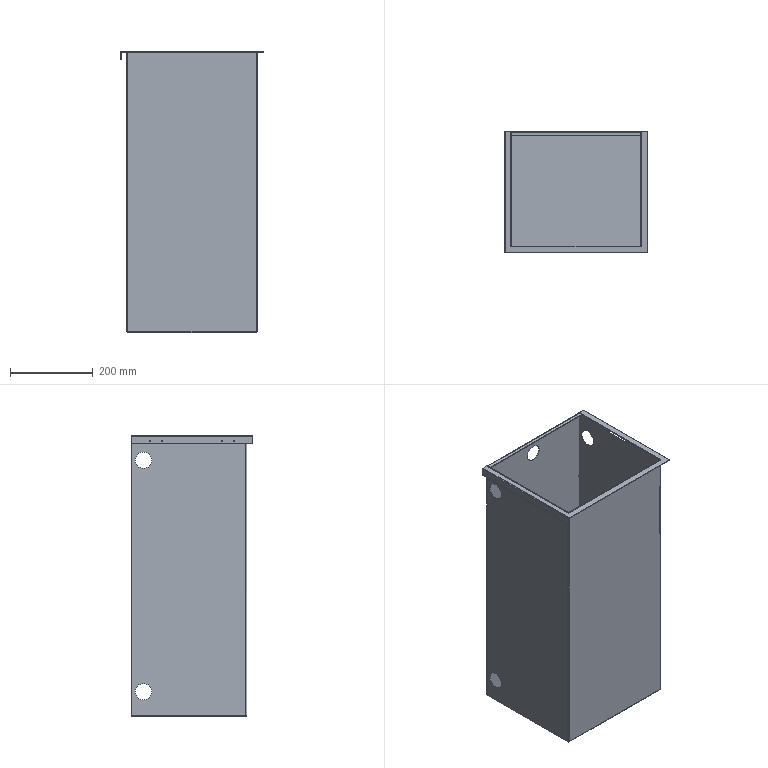Part | SolidWorks | features SMBaseFlange 5, EdgeFlange 4, FlatPattern 3, HoleWzd 3, ICE 3, SheetMetal 3, BreakCorner 1, Cut 1, Fillet 1 | 3 solids | 86 faces | box 346 x 295 x 680 mm | volume 1461449 mm3 | plane 52 | cylinder 30 | spline 4 | commonest cylinder face diameters 40 x12 3.3 x8 1.473 x5 4.473 x4 5.473 x1